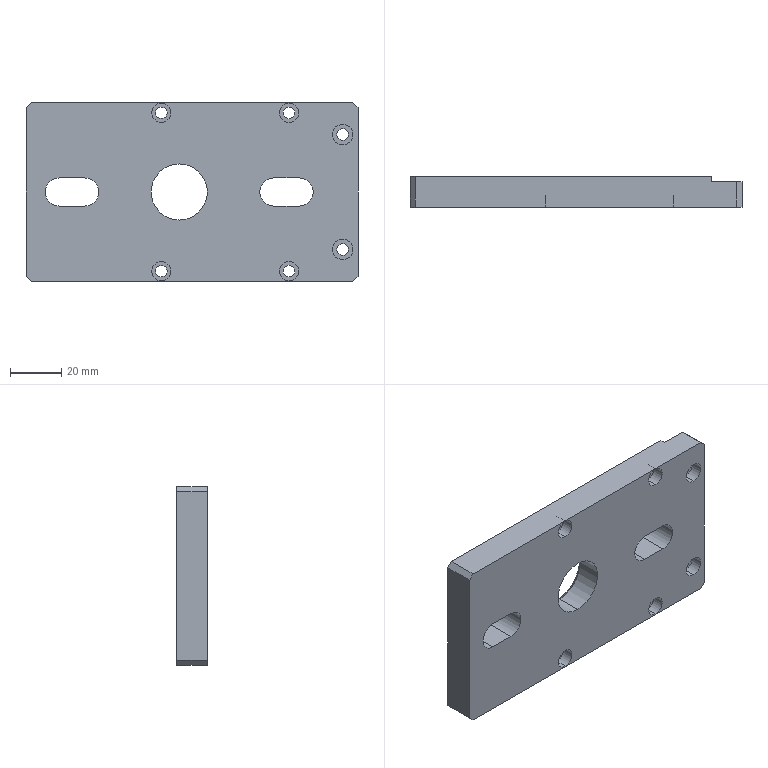Part | SolidWorks | features BaseBody 1 | 1 solid | 54 faces | box 130 x 12 x 70 mm | volume 95885 mm3 | cylinder 30 | plane 22 | cone 2 | commonest cylinder face diameters 4.5 x12 7.5 x8 8 x4 11 x4 22 x2